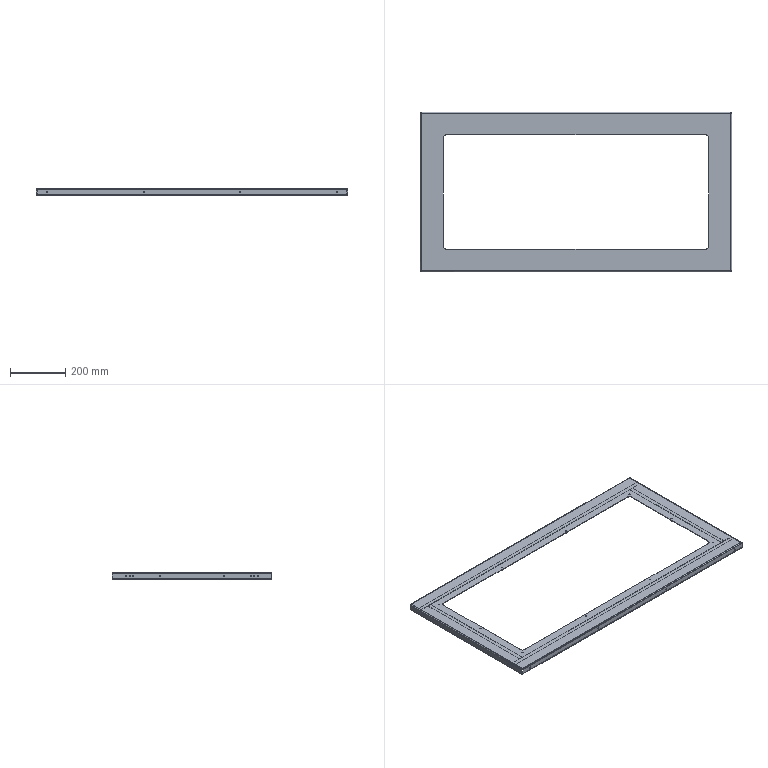Part | NX | features BREP 5 | 5 solids | 256 faces | box 1130 x 580 x 25 mm | volume 936064 mm3 | plane 124 | cylinder 96 | cone 20 | spline 16 | commonest cylinder face diameters 4.2 x24 5 x20 3.3 x16 4 x16 7 x8 8 x8